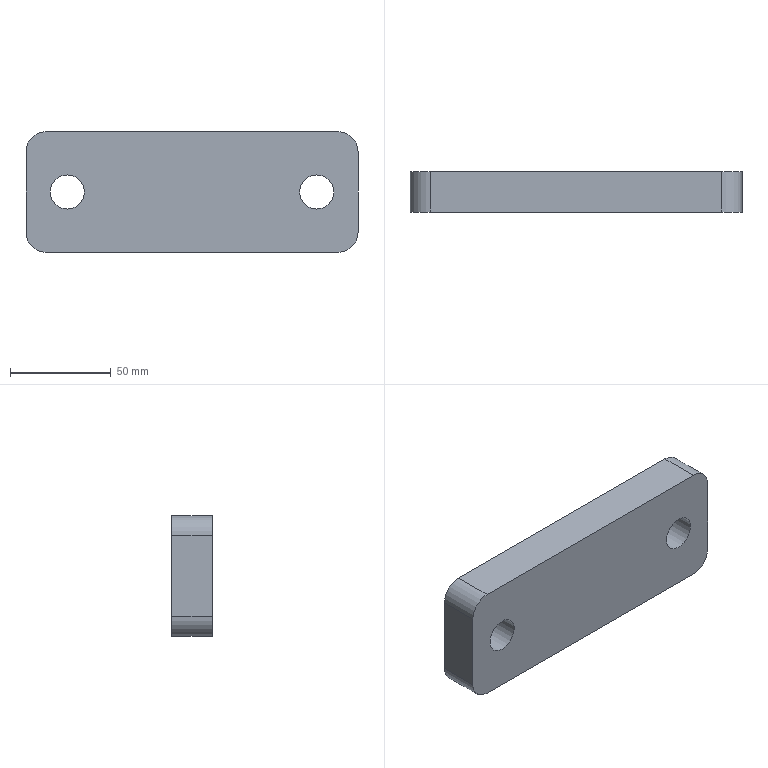Part | STEP file | JBJ-P-1000-03 | 1 solid | 12 faces | box 165 x 20 x 60 mm | volume 187204 mm3 | plane 6 | cylinder 6 | commonest cylinder face diameters 20 x4 17 x2
STEP:
#1=CARTESIAN_POINT('',(0.,20.,10.));
#2=VERTEX_POINT('',#1);
#3=CARTESIAN_POINT('',(0.,20.,50.));
#4=VERTEX_POINT('',#3);
#5=CARTESIAN_POINT('',(0.,20.,0.));
#6=DIRECTION('',(0.,0.,1.));
#7=VECTOR('',#6,1000.);
#8=LINE('',#5,#7);
#9=EDGE_CURVE('',#2,#4,#8,.T.);
#10=ORIENTED_EDGE('',*,*,#9,.F.);
#11=CARTESIAN_POINT('',(0.,0.,10.));
#12=VERTEX_POINT('',#11);
#13=CARTESIAN_POINT('',(0.,20.,10.));
#14=DIRECTION('',(0.,-1.,0.));
#15=VECTOR('',#14,1000.);
#16=LINE('',#13,#15);
#17=EDGE_CURVE('',#2,#12,#16,.T.);
#18=ORIENTED_EDGE('',*,*,#17,.T.);
#19=CARTESIAN_POINT('',(0.,0.,50.));
#20=VERTEX_POINT('',#19);
#21=CARTESIAN_POINT('',(0.,0.,0.));
#22=DIRECTION('',(0.,0.,1.));
#23=VECTOR('',#22,1000.);
#24=LINE('',#21,#23);
#25=EDGE_CURVE('',#12,#20,#24,.T.);
#26=ORIENTED_EDGE('',*,*,#25,.T.);
#27=CARTESIAN_POINT('',(0.,20.,50.));
#28=DIRECTION('',(0.,1.,0.));
#29=VECTOR('',#28,1000.);
#30=LINE('',#27,#29);
#31=EDGE_CURVE('',#20,#4,#30,.T.);
#32=ORIENTED_EDGE('',*,*,#31,.T.);
#33=EDGE_LOOP('',(#10,#18,#26,#32));
#34=FACE_OUTER_BOUND('',#33,.T.);
#35=CARTESIAN_POINT('',(0.,20.,0.));
#36=DIRECTION('',(1.,0.,0.));
#37=DIRECTION('',(0.,0.,-1.));
#38=AXIS2_PLACEMENT_3D('',#35,#36,#37);
#39=PLANE('',#38);
#40=ADVANCED_FACE('',(#34),#39,.F.);
#41=CARTESIAN_POINT('',(10.,0.,60.));
#42=VERTEX_POINT('',#41);
#43=CARTESIAN_POINT('',(155.,0.,60.));
#44=VERTEX_POINT('',#43);
#45=CARTESIAN_POINT('',(0.,0.,60.));
#46=DIRECTION('',(1.,0.,0.));
#47=VECTOR('',#46,1000.);
#48=LINE('',#45,#47);
#49=EDGE_CURVE('',#42,#44,#48,.T.);
#50=ORIENTED_EDGE('',*,*,#49,.T.);
#51=CARTESIAN_POINT('',(155.,20.,60.));
#52=VERTEX_POINT('',#51);
#53=CARTESIAN_POINT('',(155.,20.,60.));
#54=DIRECTION('',(0.,1.,0.));
#55=VECTOR('',#54,1000.);
#56=LINE('',#53,#55);
#57=EDGE_CURVE('',#44,#52,#56,.T.);
#58=ORIENTED_EDGE('',*,*,#57,.T.);
#59=CARTESIAN_POINT('',(10.,20.,60.));
#60=VERTEX_POINT('',#59);
#61=CARTESIAN_POINT('',(0.,20.,60.));
#62=DIRECTION('',(1.,0.,0.));
#63=VECTOR('',#62,1000.);
#64=LINE('',#61,#63);
#65=EDGE_CURVE('',#60,#52,#64,.T.);
#66=ORIENTED_EDGE('',*,*,#65,.F.);
#67=CARTESIAN_POINT('',(10.,20.,60.));
#68=DIRECTION('',(0.,-1.,0.));
#69=VECTOR('',#68,1000.);
#70=LINE('',#67,#69);
#71=EDGE_CURVE('',#60,#42,#70,.T.);
#72=ORIENTED_EDGE('',*,*,#71,.T.);
#73=EDGE_LOOP('',(#50,#58,#66,#72));
#74=FACE_OUTER_BOUND('',#73,.T.);
#75=CARTESIAN_POINT('',(0.,20.,60.));
#76=DIRECTION('',(0.,0.,-1.));
#77=DIRECTION('',(-1.,0.,0.));
#78=AXIS2_PLACEMENT_3D('',#75,#76,#77);
#79=PLANE('',#78);
#80=ADVANCED_FACE('',(#74),#79,.F.);
#81=CARTESIAN_POINT('',(165.,20.,50.));
#82=VERTEX_POINT('',#81);
#83=CARTESIAN_POINT('',(165.,20.,10.));
#84=VERTEX_POINT('',#83);
#85=CARTESIAN_POINT('',(165.,20.,0.));
#86=DIRECTION('',(0.,0.,-1.));
#87=VECTOR('',#86,1000.);
#88=LINE('',#85,#87);
#89=EDGE_CURVE('',#82,#84,#88,.T.);
#90=ORIENTED_EDGE('',*,*,#89,.F.);
#91=CARTESIAN_POINT('',(165.,0.,50.));
#92=VERTEX_POINT('',#91);
#93=CARTESIAN_POINT('',(165.,20.,50.));
#94=DIRECTION('',(0.,-1.,0.));
#95=VECTOR('',#94,1000.);
#96=LINE('',#93,#95);
#97=EDGE_CURVE('',#82,#92,#96,.T.);
#98=ORIENTED_EDGE('',*,*,#97,.T.);
#99=CARTESIAN_POINT('',(165.,0.,10.));
#100=VERTEX_POINT('',#99);
#101=CARTESIAN_POINT('',(165.,0.,0.));
#102=DIRECTION('',(0.,0.,-1.));
#103=VECTOR('',#102,1000.);
#104=LINE('',#101,#103);
#105=EDGE_CURVE('',#92,#100,#104,.T.);
#106=ORIENTED_EDGE('',*,*,#105,.T.);
#107=CARTESIAN_POINT('',(165.,20.,10.));
#108=DIRECTION('',(0.,1.,0.));
#109=VECTOR('',#108,1000.);
#110=LINE('',#107,#109);
#111=EDGE_CURVE('',#100,#84,#110,.T.);
#112=ORIENTED_EDGE('',*,*,#111,.T.);
#113=EDGE_LOOP('',(#90,#98,#106,#112));
#114=FACE_OUTER_BOUND('',#113,.T.);
#115=CARTESIAN_POINT('',(165.,20.,0.));
#116=DIRECTION('',(-1.,0.,0.));
#117=DIRECTION('',(0.,0.,1.));
#118=AXIS2_PLACEMENT_3D('',#115,#116,#117);
#119=PLANE('',#118);
#120=ADVANCED_FACE('',(#114),#119,.F.);
#121=CARTESIAN_POINT('',(155.,20.,0.));
#122=VERTEX_POINT('',#121);
#123=CARTESIAN_POINT('',(10.,20.,0.));
#124=VERTEX_POINT('',#123);
#125=CARTESIAN_POINT('',(0.,20.,0.));
#126=DIRECTION('',(-1.,0.,0.));
#127=VECTOR('',#126,1000.);
#128=LINE('',#125,#127);
#129=EDGE_CURVE('',#122,#124,#128,.T.);
#130=ORIENTED_EDGE('',*,*,#129,.F.);
#131=CARTESIAN_POINT('',(155.,0.,0.));
#132=VERTEX_POINT('',#131);
#133=CARTESIAN_POINT('',(155.,20.,0.));
#134=DIRECTION('',(0.,-1.,0.));
#135=VECTOR('',#134,1000.);
#136=LINE('',#133,#135);
#137=EDGE_CURVE('',#122,#132,#136,.T.);
#138=ORIENTED_EDGE('',*,*,#137,.T.);
#139=CARTESIAN_POINT('',(10.,0.,0.));
#140=VERTEX_POINT('',#139);
#141=CARTESIAN_POINT('',(0.,0.,0.));
#142=DIRECTION('',(-1.,0.,0.));
#143=VECTOR('',#142,1000.);
#144=LINE('',#141,#143);
#145=EDGE_CURVE('',#132,#140,#144,.T.);
#146=ORIENTED_EDGE('',*,*,#145,.T.);
#147=CARTESIAN_POINT('',(10.,20.,0.));
#148=DIRECTION('',(0.,1.,0.));
#149=VECTOR('',#148,1000.);
#150=LINE('',#147,#149);
#151=EDGE_CURVE('',#140,#124,#150,.T.);
#152=ORIENTED_EDGE('',*,*,#151,.T.);
#153=EDGE_LOOP('',(#130,#138,#146,#152));
#154=FACE_OUTER_BOUND('',#153,.T.);
#155=CARTESIAN_POINT('',(0.,20.,0.));
#156=DIRECTION('',(0.,0.,1.));
#157=DIRECTION('',(1.,0.,0.));
#158=AXIS2_PLACEMENT_3D('',#155,#156,#157);
#159=PLANE('',#158);
#160=ADVANCED_FACE('',(#154),#159,.F.);
#161=CARTESIAN_POINT('',(20.5,20.,38.5));
#162=VERTEX_POINT('',#161);
#163=CARTESIAN_POINT('',(20.5,20.,30.));
#164=DIRECTION('',(0.,1.,0.));
#165=DIRECTION('',(0.,0.,1.));
#166=AXIS2_PLACEMENT_3D('',#163,#164,#165);
#167=CIRCLE('',#166,8.5);
#168=EDGE_CURVE('',#162,#162,#167,.T.);
#169=ORIENTED_EDGE('',*,*,#168,.F.);
#170=EDGE_LOOP('',(#169));
#171=FACE_BOUND('',#170,.T.);
#172=CARTESIAN_POINT('',(144.5,20.,38.5));
#173=VERTEX_POINT('',#172);
#174=CARTESIAN_POINT('',(144.5,20.,30.));
#175=DIRECTION('',(0.,1.,0.));
#176=DIRECTION('',(0.,0.,1.));
#177=AXIS2_PLACEMENT_3D('',#174,#175,#176);
#178=CIRCLE('',#177,8.5);
#179=EDGE_CURVE('',#173,#173,#178,.T.);
#180=ORIENTED_EDGE('',*,*,#179,.F.);
#181=EDGE_LOOP('',(#180));
#182=FACE_BOUND('',#181,.T.);
#183=ORIENTED_EDGE('',*,*,#65,.T.);
#184=CARTESIAN_POINT('',(155.,20.,50.));
#185=DIRECTION('',(0.,1.,0.));
#186=DIRECTION('',(0.,0.,1.));
#187=AXIS2_PLACEMENT_3D('',#184,#185,#186);
#188=CIRCLE('',#187,10.);
#189=EDGE_CURVE('',#52,#82,#188,.T.);
#190=ORIENTED_EDGE('',*,*,#189,.T.);
#191=ORIENTED_EDGE('',*,*,#89,.T.);
#192=CARTESIAN_POINT('',(155.,20.,10.));
#193=DIRECTION('',(0.,1.,0.));
#194=DIRECTION('',(0.,0.,1.));
#195=AXIS2_PLACEMENT_3D('',#192,#193,#194);
#196=CIRCLE('',#195,10.);
#197=EDGE_CURVE('',#84,#122,#196,.T.);
#198=ORIENTED_EDGE('',*,*,#197,.T.);
#199=ORIENTED_EDGE('',*,*,#129,.T.);
#200=CARTESIAN_POINT('',(10.,20.,10.));
#201=DIRECTION('',(0.,1.,0.));
#202=DIRECTION('',(0.,0.,1.));
#203=AXIS2_PLACEMENT_3D('',#200,#201,#202);
#204=CIRCLE('',#203,10.);
#205=EDGE_CURVE('',#124,#2,#204,.T.);
#206=ORIENTED_EDGE('',*,*,#205,.T.);
#207=ORIENTED_EDGE('',*,*,#9,.T.);
#208=CARTESIAN_POINT('',(10.,20.,50.));
#209=DIRECTION('',(0.,1.,0.));
#210=DIRECTION('',(0.,0.,1.));
#211=AXIS2_PLACEMENT_3D('',#208,#209,#210);
#212=CIRCLE('',#211,10.);
#213=EDGE_CURVE('',#4,#60,#212,.T.);
#214=ORIENTED_EDGE('',*,*,#213,.T.);
#215=EDGE_LOOP('',(#183,#190,#191,#198,#199,#206,#207,#214));
#216=FACE_OUTER_BOUND('',#215,.T.);
#217=CARTESIAN_POINT('',(0.,20.,0.));
#218=DIRECTION('',(0.,1.,0.));
#219=DIRECTION('',(0.,0.,1.));
#220=AXIS2_PLACEMENT_3D('',#217,#218,#219);
#221=PLANE('',#220);
#222=ADVANCED_FACE('',(#171,#182,#216),#221,.T.);
#223=CARTESIAN_POINT('',(20.5,0.,38.5));
#224=VERTEX_POINT('',#223);
#225=CARTESIAN_POINT('',(20.5,0.,30.));
#226=DIRECTION('',(0.,1.,0.));
#227=DIRECTION('',(0.,0.,1.));
#228=AXIS2_PLACEMENT_3D('',#225,#226,#227);
#229=CIRCLE('',#228,8.5);
#230=EDGE_CURVE('',#224,#224,#229,.T.);
#231=ORIENTED_EDGE('',*,*,#230,.T.);
#232=EDGE_LOOP('',(#231));
#233=FACE_BOUND('',#232,.T.);
#234=CARTESIAN_POINT('',(144.5,0.,38.5));
#235=VERTEX_POINT('',#234);
#236=CARTESIAN_POINT('',(144.5,0.,30.));
#237=DIRECTION('',(0.,1.,0.));
#238=DIRECTION('',(0.,0.,1.));
#239=AXIS2_PLACEMENT_3D('',#236,#237,#238);
#240=CIRCLE('',#239,8.5);
#241=EDGE_CURVE('',#235,#235,#240,.T.);
#242=ORIENTED_EDGE('',*,*,#241,.T.);
#243=EDGE_LOOP('',(#242));
#244=FACE_BOUND('',#243,.T.);
#245=ORIENTED_EDGE('',*,*,#105,.F.);
#246=CARTESIAN_POINT('',(155.,0.,50.));
#247=DIRECTION('',(0.,-1.,0.));
#248=DIRECTION('',(0.,0.,1.));
#249=AXIS2_PLACEMENT_3D('',#246,#247,#248);
#250=CIRCLE('',#249,10.);
#251=EDGE_CURVE('',#92,#44,#250,.T.);
#252=ORIENTED_EDGE('',*,*,#251,.T.);
#253=ORIENTED_EDGE('',*,*,#49,.F.);
#254=CARTESIAN_POINT('',(10.,0.,50.));
#255=DIRECTION('',(0.,-1.,0.));
#256=DIRECTION('',(0.,0.,1.));
#257=AXIS2_PLACEMENT_3D('',#254,#255,#256);
#258=CIRCLE('',#257,10.);
#259=EDGE_CURVE('',#42,#20,#258,.T.);
#260=ORIENTED_EDGE('',*,*,#259,.T.);
#261=ORIENTED_EDGE('',*,*,#25,.F.);
#262=CARTESIAN_POINT('',(10.,0.,10.));
#263=DIRECTION('',(0.,-1.,0.));
#264=DIRECTION('',(0.,0.,1.));
#265=AXIS2_PLACEMENT_3D('',#262,#263,#264);
#266=CIRCLE('',#265,10.);
#267=EDGE_CURVE('',#12,#140,#266,.T.);
#268=ORIENTED_EDGE('',*,*,#267,.T.);
#269=ORIENTED_EDGE('',*,*,#145,.F.);
#270=CARTESIAN_POINT('',(155.,0.,10.));
#271=DIRECTION('',(0.,-1.,0.));
#272=DIRECTION('',(0.,0.,1.));
#273=AXIS2_PLACEMENT_3D('',#270,#271,#272);
#274=CIRCLE('',#273,10.);
#275=EDGE_CURVE('',#132,#100,#274,.T.);
#276=ORIENTED_EDGE('',*,*,#275,.T.);
#277=EDGE_LOOP('',(#245,#252,#253,#260,#261,#268,#269,#276));
#278=FACE_OUTER_BOUND('',#277,.T.);
#279=CARTESIAN_POINT('',(0.,0.,0.));
#280=DIRECTION('',(0.,1.,0.));
#281=DIRECTION('',(0.,0.,1.));
#282=AXIS2_PLACEMENT_3D('',#279,#280,#281);
#283=PLANE('',#282);
#284=ADVANCED_FACE('',(#233,#244,#278),#283,.F.);
#285=ORIENTED_EDGE('',*,*,#179,.T.);
#286=EDGE_LOOP('',(#285));
#287=FACE_OUTER_BOUND('',#286,.T.);
#288=ORIENTED_EDGE('',*,*,#241,.F.);
#289=EDGE_LOOP('',(#288));
#290=FACE_OUTER_BOUND('',#289,.T.);
#291=CARTESIAN_POINT('',(144.5,20.,30.));
#292=DIRECTION('',(0.,1.,0.));
#293=DIRECTION('',(0.,0.,1.));
#294=AXIS2_PLACEMENT_3D('',#291,#292,#293);
#295=CYLINDRICAL_SURFACE('',#294,8.5);
#296=ADVANCED_FACE('',(#287,#290),#295,.F.);
#297=ORIENTED_EDGE('',*,*,#168,.T.);
#298=EDGE_LOOP('',(#297));
#299=FACE_OUTER_BOUND('',#298,.T.);
#300=ORIENTED_EDGE('',*,*,#230,.F.);
#301=EDGE_LOOP('',(#300));
#302=FACE_OUTER_BOUND('',#301,.T.);
#303=CARTESIAN_POINT('',(20.5,20.,30.));
#304=DIRECTION('',(0.,1.,0.));
#305=DIRECTION('',(0.,0.,1.));
#306=AXIS2_PLACEMENT_3D('',#303,#304,#305);
#307=CYLINDRICAL_SURFACE('',#306,8.5);
#308=ADVANCED_FACE('',(#299,#302),#307,.F.);
#309=ORIENTED_EDGE('',*,*,#189,.F.);
#310=ORIENTED_EDGE('',*,*,#57,.F.);
#311=ORIENTED_EDGE('',*,*,#251,.F.);
#312=ORIENTED_EDGE('',*,*,#97,.F.);
#313=EDGE_LOOP('',(#309,#310,#311,#312));
#314=FACE_OUTER_BOUND('',#313,.T.);
#315=CARTESIAN_POINT('',(155.,20.,50.));
#316=DIRECTION('',(0.,-1.,0.));
#317=DIRECTION('',(0.,0.,-1.));
#318=AXIS2_PLACEMENT_3D('',#315,#316,#317);
#319=CYLINDRICAL_SURFACE('',#318,10.);
#320=ADVANCED_FACE('',(#314),#319,.T.);
#321=ORIENTED_EDGE('',*,*,#197,.F.);
#322=ORIENTED_EDGE('',*,*,#111,.F.);
#323=ORIENTED_EDGE('',*,*,#275,.F.);
#324=ORIENTED_EDGE('',*,*,#137,.F.);
#325=EDGE_LOOP('',(#321,#322,#323,#324));
#326=FACE_OUTER_BOUND('',#325,.T.);
#327=CARTESIAN_POINT('',(155.,20.,10.));
#328=DIRECTION('',(0.,-1.,0.));
#329=DIRECTION('',(0.,0.,-1.));
#330=AXIS2_PLACEMENT_3D('',#327,#328,#329);
#331=CYLINDRICAL_SURFACE('',#330,10.);
#332=ADVANCED_FACE('',(#326),#331,.T.);
#333=ORIENTED_EDGE('',*,*,#205,.F.);
#334=ORIENTED_EDGE('',*,*,#151,.F.);
#335=ORIENTED_EDGE('',*,*,#267,.F.);
#336=ORIENTED_EDGE('',*,*,#17,.F.);
#337=EDGE_LOOP('',(#333,#334,#335,#336));
#338=FACE_OUTER_BOUND('',#337,.T.);
#339=CARTESIAN_POINT('',(10.,20.,10.));
#340=DIRECTION('',(0.,-1.,0.));
#341=DIRECTION('',(0.,0.,-1.));
#342=AXIS2_PLACEMENT_3D('',#339,#340,#341);
#343=CYLINDRICAL_SURFACE('',#342,10.);
#344=ADVANCED_FACE('',(#338),#343,.T.);
#345=ORIENTED_EDGE('',*,*,#213,.F.);
#346=ORIENTED_EDGE('',*,*,#31,.F.);
#347=ORIENTED_EDGE('',*,*,#259,.F.);
#348=ORIENTED_EDGE('',*,*,#71,.F.);
#349=EDGE_LOOP('',(#345,#346,#347,#348));
#350=FACE_OUTER_BOUND('',#349,.T.);
#351=CARTESIAN_POINT('',(10.,20.,50.));
#352=DIRECTION('',(0.,-1.,0.));
#353=DIRECTION('',(0.,0.,-1.));
#354=AXIS2_PLACEMENT_3D('',#351,#352,#353);
#355=CYLINDRICAL_SURFACE('',#354,10.);
#356=ADVANCED_FACE('',(#350),#355,.T.);
#357=CLOSED_SHELL('',(#40,#80,#120,#160,#222,#284,#296,#308,#320,#332,#344,#356));
#358=MANIFOLD_SOLID_BREP('',#357);
#359=CARTESIAN_POINT('',(0.,0.,0.));
#360=DIRECTION('',(0.,0.,1.));
#361=DIRECTION('',(1.,0.,0.));
#362=AXIS2_PLACEMENT_3D('',#359,#360,#361);
#363=(LENGTH_UNIT()NAMED_UNIT(*)SI_UNIT(.MILLI.,.METRE.));
#364=UNCERTAINTY_MEASURE_WITH_UNIT(LENGTH_MEASURE(0.00001),#363,'','');
#365=(NAMED_UNIT(*)PLANE_ANGLE_UNIT()SI_UNIT($,.RADIAN.));
#366=(NAMED_UNIT(*)SI_UNIT($,.STERADIAN.)SOLID_ANGLE_UNIT());
#367=(GEOMETRIC_REPRESENTATION_CONTEXT(3)GLOBAL_UNCERTAINTY_ASSIGNED_CONTEXT((#364))GLOBAL_UNIT_ASSIGNED_CONTEXT((#363,#365,#366))REPRESENTATION_CONTEXT('',''));
#368=ADVANCED_BREP_SHAPE_REPRESENTATION('',(#358,#362),#367);